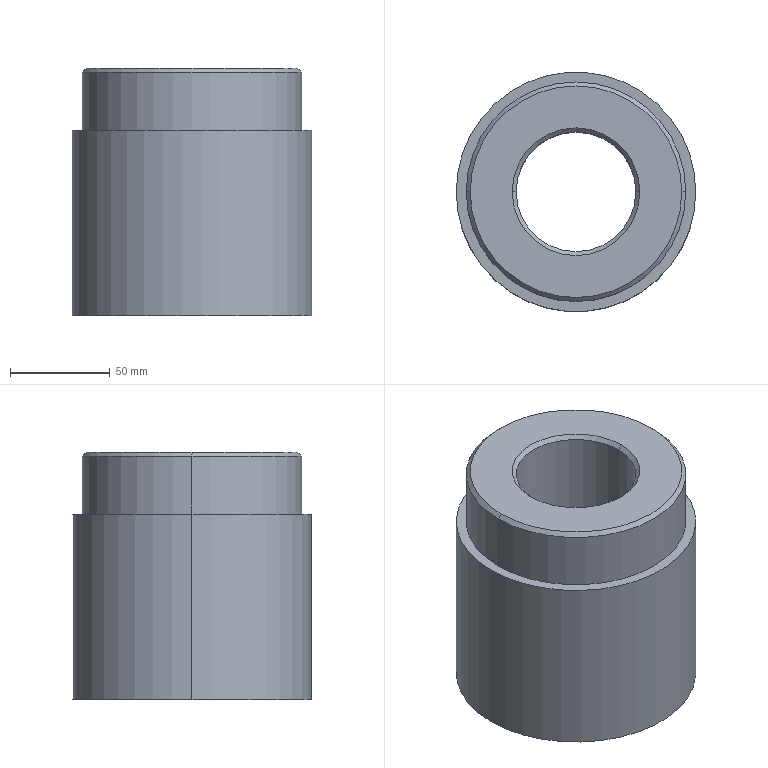Part | SolidWorks | features Chamfer 1, Extrusion 1, ICE 1 | 1 solid | 15 faces | box 120 x 120 x 124 mm | volume 994353 mm3 | cone 6 | cylinder 6 | plane 3 | commonest cylinder face diameters 60 x2 110 x2 120 x2
STEP:
#1=CARTESIAN_POINT('',(-30.,0.,122.));
#2=VERTEX_POINT('',#1);
#3=CARTESIAN_POINT('',(30.,0.,122.));
#4=VERTEX_POINT('',#3);
#5=CARTESIAN_POINT('',(0.,0.,122.));
#6=DIRECTION('',(0.,0.,1.));
#7=DIRECTION('',(1.,0.,0.));
#8=AXIS2_PLACEMENT_3D('',#5,#6,#7);
#9=CIRCLE('',#8,30.);
#10=EDGE_CURVE('',#2,#4,#9,.T.);
#11=ORIENTED_EDGE('',*,*,#10,.F.);
#12=CARTESIAN_POINT('',(-32.,0.,124.));
#13=VERTEX_POINT('',#12);
#14=CARTESIAN_POINT('',(-30.,0.,122.));
#15=DIRECTION('',(-0.7071,0.,0.7071));
#16=VECTOR('',#15,1000.);
#17=LINE('',#14,#16);
#18=EDGE_CURVE('',#2,#13,#17,.T.);
#19=ORIENTED_EDGE('',*,*,#18,.T.);
#20=CARTESIAN_POINT('',(32.,0.,124.));
#21=VERTEX_POINT('',#20);
#22=CARTESIAN_POINT('',(0.,0.,124.));
#23=DIRECTION('',(0.,0.,-1.));
#24=DIRECTION('',(1.,0.,0.));
#25=AXIS2_PLACEMENT_3D('',#22,#23,#24);
#26=CIRCLE('',#25,32.);
#27=EDGE_CURVE('',#21,#13,#26,.T.);
#28=ORIENTED_EDGE('',*,*,#27,.F.);
#29=CARTESIAN_POINT('',(30.,0.,122.));
#30=DIRECTION('',(0.7071,0.,0.7071));
#31=VECTOR('',#30,1000.);
#32=LINE('',#29,#31);
#33=EDGE_CURVE('',#4,#21,#32,.T.);
#34=ORIENTED_EDGE('',*,*,#33,.F.);
#35=EDGE_LOOP('',(#11,#19,#28,#34));
#36=FACE_OUTER_BOUND('',#35,.T.);
#37=CARTESIAN_POINT('',(0.,0.,122.));
#38=DIRECTION('',(0.,0.,1.));
#39=DIRECTION('',(1.,0.,0.));
#40=AXIS2_PLACEMENT_3D('',#37,#38,#39);
#41=CONICAL_SURFACE('',#40,30.,0.7854);
#42=ADVANCED_FACE('',(#36),#41,.F.);
#43=CARTESIAN_POINT('',(53.,0.,124.));
#44=VERTEX_POINT('',#43);
#45=CARTESIAN_POINT('',(-53.,0.,124.));
#46=VERTEX_POINT('',#45);
#47=CARTESIAN_POINT('',(0.,0.,124.));
#48=DIRECTION('',(0.,0.,1.));
#49=DIRECTION('',(1.,0.,0.));
#50=AXIS2_PLACEMENT_3D('',#47,#48,#49);
#51=CIRCLE('',#50,53.);
#52=EDGE_CURVE('',#44,#46,#51,.T.);
#53=ORIENTED_EDGE('',*,*,#52,.F.);
#54=CARTESIAN_POINT('',(55.,0.,122.));
#55=VERTEX_POINT('',#54);
#56=CARTESIAN_POINT('',(53.,0.,124.));
#57=DIRECTION('',(0.7071,0.,-0.7071));
#58=VECTOR('',#57,1000.);
#59=LINE('',#56,#58);
#60=EDGE_CURVE('',#44,#55,#59,.T.);
#61=ORIENTED_EDGE('',*,*,#60,.T.);
#62=CARTESIAN_POINT('',(-55.,0.,122.));
#63=VERTEX_POINT('',#62);
#64=CARTESIAN_POINT('',(0.,0.,122.));
#65=DIRECTION('',(0.,0.,-1.));
#66=DIRECTION('',(1.,0.,0.));
#67=AXIS2_PLACEMENT_3D('',#64,#65,#66);
#68=CIRCLE('',#67,55.);
#69=EDGE_CURVE('',#63,#55,#68,.T.);
#70=ORIENTED_EDGE('',*,*,#69,.F.);
#71=CARTESIAN_POINT('',(-53.,0.,124.));
#72=DIRECTION('',(-0.7071,0.,-0.7071));
#73=VECTOR('',#72,1000.);
#74=LINE('',#71,#73);
#75=EDGE_CURVE('',#46,#63,#74,.T.);
#76=ORIENTED_EDGE('',*,*,#75,.F.);
#77=EDGE_LOOP('',(#53,#61,#70,#76));
#78=FACE_OUTER_BOUND('',#77,.T.);
#79=CARTESIAN_POINT('',(0.,0.,124.));
#80=DIRECTION('',(0.,0.,-1.));
#81=DIRECTION('',(-1.,0.,0.));
#82=AXIS2_PLACEMENT_3D('',#79,#80,#81);
#83=CONICAL_SURFACE('',#82,53.,0.7854);
#84=ADVANCED_FACE('',(#78),#83,.T.);
#85=CARTESIAN_POINT('',(30.,0.,2.));
#86=VERTEX_POINT('',#85);
#87=CARTESIAN_POINT('',(-30.,0.,2.));
#88=VERTEX_POINT('',#87);
#89=CARTESIAN_POINT('',(0.,0.,2.));
#90=DIRECTION('',(0.,0.,-1.));
#91=DIRECTION('',(1.,0.,0.));
#92=AXIS2_PLACEMENT_3D('',#89,#90,#91);
#93=CIRCLE('',#92,30.);
#94=EDGE_CURVE('',#86,#88,#93,.T.);
#95=ORIENTED_EDGE('',*,*,#94,.F.);
#96=CARTESIAN_POINT('',(32.,0.,0.));
#97=VERTEX_POINT('',#96);
#98=CARTESIAN_POINT('',(32.,0.,0.));
#99=DIRECTION('',(0.7071,0.,-0.7071));
#100=VECTOR('',#99,1000.);
#101=LINE('',#98,#100);
#102=EDGE_CURVE('',#86,#97,#101,.T.);
#103=ORIENTED_EDGE('',*,*,#102,.T.);
#104=CARTESIAN_POINT('',(-32.,0.,0.));
#105=VERTEX_POINT('',#104);
#106=CARTESIAN_POINT('',(0.,0.,0.));
#107=DIRECTION('',(0.,0.,1.));
#108=DIRECTION('',(1.,0.,0.));
#109=AXIS2_PLACEMENT_3D('',#106,#107,#108);
#110=CIRCLE('',#109,32.);
#111=EDGE_CURVE('',#105,#97,#110,.T.);
#112=ORIENTED_EDGE('',*,*,#111,.F.);
#113=CARTESIAN_POINT('',(-32.,0.,0.));
#114=DIRECTION('',(-0.7071,0.,-0.7071));
#115=VECTOR('',#114,1000.);
#116=LINE('',#113,#115);
#117=EDGE_CURVE('',#88,#105,#116,.T.);
#118=ORIENTED_EDGE('',*,*,#117,.F.);
#119=EDGE_LOOP('',(#95,#103,#112,#118));
#120=FACE_OUTER_BOUND('',#119,.T.);
#121=CARTESIAN_POINT('',(0.,0.,0.));
#122=DIRECTION('',(0.,0.,-1.));
#123=DIRECTION('',(-1.,0.,0.));
#124=AXIS2_PLACEMENT_3D('',#121,#122,#123);
#125=CONICAL_SURFACE('',#124,32.,0.7854);
#126=ADVANCED_FACE('',(#120),#125,.F.);
#127=CARTESIAN_POINT('',(55.,0.,93.));
#128=VERTEX_POINT('',#127);
#129=CARTESIAN_POINT('',(-55.,0.,93.));
#130=VERTEX_POINT('',#129);
#131=CARTESIAN_POINT('',(0.,0.,93.));
#132=DIRECTION('',(0.,0.,1.));
#133=DIRECTION('',(1.,0.,0.));
#134=AXIS2_PLACEMENT_3D('',#131,#132,#133);
#135=CIRCLE('',#134,55.);
#136=EDGE_CURVE('',#128,#130,#135,.T.);
#137=ORIENTED_EDGE('',*,*,#136,.T.);
#138=CARTESIAN_POINT('',(-55.,0.,93.));
#139=DIRECTION('',(0.,0.,1.));
#140=VECTOR('',#139,1000.);
#141=LINE('',#138,#140);
#142=EDGE_CURVE('',#130,#63,#141,.T.);
#143=ORIENTED_EDGE('',*,*,#142,.T.);
#144=ORIENTED_EDGE('',*,*,#69,.T.);
#145=CARTESIAN_POINT('',(55.,0.,93.));
#146=DIRECTION('',(0.,0.,1.));
#147=VECTOR('',#146,1000.);
#148=LINE('',#145,#147);
#149=EDGE_CURVE('',#128,#55,#148,.T.);
#150=ORIENTED_EDGE('',*,*,#149,.F.);
#151=EDGE_LOOP('',(#137,#143,#144,#150));
#152=FACE_OUTER_BOUND('',#151,.T.);
#153=CARTESIAN_POINT('',(0.,0.,93.));
#154=DIRECTION('',(0.,0.,1.));
#155=DIRECTION('',(1.,0.,0.));
#156=AXIS2_PLACEMENT_3D('',#153,#154,#155);
#157=CYLINDRICAL_SURFACE('',#156,55.);
#158=ADVANCED_FACE('',(#152),#157,.T.);
#159=ORIENTED_EDGE('',*,*,#10,.T.);
#160=CARTESIAN_POINT('',(30.,0.,124.));
#161=DIRECTION('',(0.,0.,-1.));
#162=VECTOR('',#161,1000.);
#163=LINE('',#160,#162);
#164=EDGE_CURVE('',#4,#86,#163,.T.);
#165=ORIENTED_EDGE('',*,*,#164,.T.);
#166=ORIENTED_EDGE('',*,*,#94,.T.);
#167=CARTESIAN_POINT('',(-30.,0.,124.));
#168=DIRECTION('',(0.,0.,-1.));
#169=VECTOR('',#168,1000.);
#170=LINE('',#167,#169);
#171=EDGE_CURVE('',#2,#88,#170,.T.);
#172=ORIENTED_EDGE('',*,*,#171,.F.);
#173=EDGE_LOOP('',(#159,#165,#166,#172));
#174=FACE_OUTER_BOUND('',#173,.T.);
#175=CARTESIAN_POINT('',(0.,0.,124.));
#176=DIRECTION('',(0.,0.,-1.));
#177=DIRECTION('',(-1.,0.,0.));
#178=AXIS2_PLACEMENT_3D('',#175,#176,#177);
#179=CYLINDRICAL_SURFACE('',#178,30.);
#180=ADVANCED_FACE('',(#174),#179,.F.);
#181=CARTESIAN_POINT('',(60.,0.,93.));
#182=VERTEX_POINT('',#181);
#183=CARTESIAN_POINT('',(-60.,0.,93.));
#184=VERTEX_POINT('',#183);
#185=CARTESIAN_POINT('',(0.,0.,93.));
#186=DIRECTION('',(0.,0.,1.));
#187=DIRECTION('',(1.,0.,0.));
#188=AXIS2_PLACEMENT_3D('',#185,#186,#187);
#189=CIRCLE('',#188,60.);
#190=EDGE_CURVE('',#182,#184,#189,.T.);
#191=ORIENTED_EDGE('',*,*,#190,.F.);
#192=CARTESIAN_POINT('',(60.,0.,0.));
#193=VERTEX_POINT('',#192);
#194=CARTESIAN_POINT('',(60.,0.,124.));
#195=DIRECTION('',(0.,0.,-1.));
#196=VECTOR('',#195,1000.);
#197=LINE('',#194,#196);
#198=EDGE_CURVE('',#182,#193,#197,.T.);
#199=ORIENTED_EDGE('',*,*,#198,.T.);
#200=CARTESIAN_POINT('',(-60.,0.,0.));
#201=VERTEX_POINT('',#200);
#202=CARTESIAN_POINT('',(0.,0.,0.));
#203=DIRECTION('',(0.,0.,1.));
#204=DIRECTION('',(1.,0.,0.));
#205=AXIS2_PLACEMENT_3D('',#202,#203,#204);
#206=CIRCLE('',#205,60.);
#207=EDGE_CURVE('',#193,#201,#206,.T.);
#208=ORIENTED_EDGE('',*,*,#207,.T.);
#209=CARTESIAN_POINT('',(-60.,0.,124.));
#210=DIRECTION('',(0.,0.,-1.));
#211=VECTOR('',#210,1000.);
#212=LINE('',#209,#211);
#213=EDGE_CURVE('',#184,#201,#212,.T.);
#214=ORIENTED_EDGE('',*,*,#213,.F.);
#215=EDGE_LOOP('',(#191,#199,#208,#214));
#216=FACE_OUTER_BOUND('',#215,.T.);
#217=CARTESIAN_POINT('',(0.,0.,124.));
#218=DIRECTION('',(0.,0.,-1.));
#219=DIRECTION('',(-1.,0.,0.));
#220=AXIS2_PLACEMENT_3D('',#217,#218,#219);
#221=CYLINDRICAL_SURFACE('',#220,60.);
#222=ADVANCED_FACE('',(#216),#221,.T.);
#223=CARTESIAN_POINT('',(0.,0.,124.));
#224=DIRECTION('',(0.,0.,1.));
#225=DIRECTION('',(1.,0.,0.));
#226=AXIS2_PLACEMENT_3D('',#223,#224,#225);
#227=CIRCLE('',#226,53.);
#228=EDGE_CURVE('',#46,#44,#227,.T.);
#229=ORIENTED_EDGE('',*,*,#228,.T.);
#230=ORIENTED_EDGE('',*,*,#52,.T.);
#231=EDGE_LOOP('',(#229,#230));
#232=FACE_OUTER_BOUND('',#231,.T.);
#233=ORIENTED_EDGE('',*,*,#27,.T.);
#234=CARTESIAN_POINT('',(0.,0.,124.));
#235=DIRECTION('',(0.,0.,-1.));
#236=DIRECTION('',(1.,0.,0.));
#237=AXIS2_PLACEMENT_3D('',#234,#235,#236);
#238=CIRCLE('',#237,32.);
#239=EDGE_CURVE('',#13,#21,#238,.T.);
#240=ORIENTED_EDGE('',*,*,#239,.T.);
#241=EDGE_LOOP('',(#233,#240));
#242=FACE_BOUND('',#241,.T.);
#243=CARTESIAN_POINT('',(0.,0.,124.));
#244=DIRECTION('',(0.,0.,1.));
#245=DIRECTION('',(1.,0.,0.));
#246=AXIS2_PLACEMENT_3D('',#243,#244,#245);
#247=PLANE('',#246);
#248=ADVANCED_FACE('',(#232,#242),#247,.T.);
#249=ORIENTED_EDGE('',*,*,#198,.F.);
#250=CARTESIAN_POINT('',(0.,0.,93.));
#251=DIRECTION('',(0.,0.,1.));
#252=DIRECTION('',(1.,0.,0.));
#253=AXIS2_PLACEMENT_3D('',#250,#251,#252);
#254=CIRCLE('',#253,60.);
#255=EDGE_CURVE('',#184,#182,#254,.T.);
#256=ORIENTED_EDGE('',*,*,#255,.F.);
#257=ORIENTED_EDGE('',*,*,#213,.T.);
#258=CARTESIAN_POINT('',(0.,0.,0.));
#259=DIRECTION('',(0.,0.,1.));
#260=DIRECTION('',(1.,0.,0.));
#261=AXIS2_PLACEMENT_3D('',#258,#259,#260);
#262=CIRCLE('',#261,60.);
#263=EDGE_CURVE('',#201,#193,#262,.T.);
#264=ORIENTED_EDGE('',*,*,#263,.T.);
#265=EDGE_LOOP('',(#249,#256,#257,#264));
#266=FACE_OUTER_BOUND('',#265,.T.);
#267=CARTESIAN_POINT('',(0.,0.,124.));
#268=DIRECTION('',(0.,0.,-1.));
#269=DIRECTION('',(-1.,0.,0.));
#270=AXIS2_PLACEMENT_3D('',#267,#268,#269);
#271=CYLINDRICAL_SURFACE('',#270,60.);
#272=ADVANCED_FACE('',(#266),#271,.T.);
#273=ORIENTED_EDGE('',*,*,#111,.T.);
#274=CARTESIAN_POINT('',(0.,0.,0.));
#275=DIRECTION('',(0.,0.,1.));
#276=DIRECTION('',(1.,0.,0.));
#277=AXIS2_PLACEMENT_3D('',#274,#275,#276);
#278=CIRCLE('',#277,32.);
#279=EDGE_CURVE('',#97,#105,#278,.T.);
#280=ORIENTED_EDGE('',*,*,#279,.T.);
#281=EDGE_LOOP('',(#273,#280));
#282=FACE_BOUND('',#281,.T.);
#283=ORIENTED_EDGE('',*,*,#263,.F.);
#284=ORIENTED_EDGE('',*,*,#207,.F.);
#285=EDGE_LOOP('',(#283,#284));
#286=FACE_OUTER_BOUND('',#285,.T.);
#287=CARTESIAN_POINT('',(0.,0.,0.));
#288=DIRECTION('',(0.,0.,1.));
#289=DIRECTION('',(1.,0.,0.));
#290=AXIS2_PLACEMENT_3D('',#287,#288,#289);
#291=PLANE('',#290);
#292=ADVANCED_FACE('',(#282,#286),#291,.F.);
#293=ORIENTED_EDGE('',*,*,#164,.F.);
#294=CARTESIAN_POINT('',(0.,0.,122.));
#295=DIRECTION('',(0.,0.,1.));
#296=DIRECTION('',(1.,0.,0.));
#297=AXIS2_PLACEMENT_3D('',#294,#295,#296);
#298=CIRCLE('',#297,30.);
#299=EDGE_CURVE('',#4,#2,#298,.T.);
#300=ORIENTED_EDGE('',*,*,#299,.T.);
#301=ORIENTED_EDGE('',*,*,#171,.T.);
#302=CARTESIAN_POINT('',(0.,0.,2.));
#303=DIRECTION('',(0.,0.,-1.));
#304=DIRECTION('',(1.,0.,0.));
#305=AXIS2_PLACEMENT_3D('',#302,#303,#304);
#306=CIRCLE('',#305,30.);
#307=EDGE_CURVE('',#88,#86,#306,.T.);
#308=ORIENTED_EDGE('',*,*,#307,.T.);
#309=EDGE_LOOP('',(#293,#300,#301,#308));
#310=FACE_OUTER_BOUND('',#309,.T.);
#311=CARTESIAN_POINT('',(0.,0.,124.));
#312=DIRECTION('',(0.,0.,-1.));
#313=DIRECTION('',(-1.,0.,0.));
#314=AXIS2_PLACEMENT_3D('',#311,#312,#313);
#315=CYLINDRICAL_SURFACE('',#314,30.);
#316=ADVANCED_FACE('',(#310),#315,.F.);
#317=ORIENTED_EDGE('',*,*,#136,.F.);
#318=CARTESIAN_POINT('',(0.,0.,93.));
#319=DIRECTION('',(0.,0.,1.));
#320=DIRECTION('',(1.,0.,0.));
#321=AXIS2_PLACEMENT_3D('',#318,#319,#320);
#322=CIRCLE('',#321,55.);
#323=EDGE_CURVE('',#130,#128,#322,.T.);
#324=ORIENTED_EDGE('',*,*,#323,.F.);
#325=EDGE_LOOP('',(#317,#324));
#326=FACE_BOUND('',#325,.T.);
#327=ORIENTED_EDGE('',*,*,#255,.T.);
#328=ORIENTED_EDGE('',*,*,#190,.T.);
#329=EDGE_LOOP('',(#327,#328));
#330=FACE_OUTER_BOUND('',#329,.T.);
#331=CARTESIAN_POINT('',(0.,0.,93.));
#332=DIRECTION('',(0.,0.,1.));
#333=DIRECTION('',(1.,0.,0.));
#334=AXIS2_PLACEMENT_3D('',#331,#332,#333);
#335=PLANE('',#334);
#336=ADVANCED_FACE('',(#326,#330),#335,.T.);
#337=ORIENTED_EDGE('',*,*,#142,.F.);
#338=ORIENTED_EDGE('',*,*,#323,.T.);
#339=ORIENTED_EDGE('',*,*,#149,.T.);
#340=CARTESIAN_POINT('',(0.,0.,122.));
#341=DIRECTION('',(0.,0.,-1.));
#342=DIRECTION('',(1.,0.,0.));
#343=AXIS2_PLACEMENT_3D('',#340,#341,#342);
#344=CIRCLE('',#343,55.);
#345=EDGE_CURVE('',#55,#63,#344,.T.);
#346=ORIENTED_EDGE('',*,*,#345,.T.);
#347=EDGE_LOOP('',(#337,#338,#339,#346));
#348=FACE_OUTER_BOUND('',#347,.T.);
#349=CARTESIAN_POINT('',(0.,0.,93.));
#350=DIRECTION('',(0.,0.,1.));
#351=DIRECTION('',(1.,0.,0.));
#352=AXIS2_PLACEMENT_3D('',#349,#350,#351);
#353=CYLINDRICAL_SURFACE('',#352,55.);
#354=ADVANCED_FACE('',(#348),#353,.T.);
#355=ORIENTED_EDGE('',*,*,#102,.F.);
#356=ORIENTED_EDGE('',*,*,#307,.F.);
#357=ORIENTED_EDGE('',*,*,#117,.T.);
#358=ORIENTED_EDGE('',*,*,#279,.F.);
#359=EDGE_LOOP('',(#355,#356,#357,#358));
#360=FACE_OUTER_BOUND('',#359,.T.);
#361=CARTESIAN_POINT('',(0.,0.,0.));
#362=DIRECTION('',(0.,0.,-1.));
#363=DIRECTION('',(-1.,0.,0.));
#364=AXIS2_PLACEMENT_3D('',#361,#362,#363);
#365=CONICAL_SURFACE('',#364,32.,0.7854);
#366=ADVANCED_FACE('',(#360),#365,.F.);
#367=ORIENTED_EDGE('',*,*,#60,.F.);
#368=ORIENTED_EDGE('',*,*,#228,.F.);
#369=ORIENTED_EDGE('',*,*,#75,.T.);
#370=ORIENTED_EDGE('',*,*,#345,.F.);
#371=EDGE_LOOP('',(#367,#368,#369,#370));
#372=FACE_OUTER_BOUND('',#371,.T.);
#373=CARTESIAN_POINT('',(0.,0.,124.));
#374=DIRECTION('',(0.,0.,-1.));
#375=DIRECTION('',(-1.,0.,0.));
#376=AXIS2_PLACEMENT_3D('',#373,#374,#375);
#377=CONICAL_SURFACE('',#376,53.,0.7854);
#378=ADVANCED_FACE('',(#372),#377,.T.);
#379=ORIENTED_EDGE('',*,*,#18,.F.);
#380=ORIENTED_EDGE('',*,*,#299,.F.);
#381=ORIENTED_EDGE('',*,*,#33,.T.);
#382=ORIENTED_EDGE('',*,*,#239,.F.);
#383=EDGE_LOOP('',(#379,#380,#381,#382));
#384=FACE_OUTER_BOUND('',#383,.T.);
#385=CARTESIAN_POINT('',(0.,0.,122.));
#386=DIRECTION('',(0.,0.,1.));
#387=DIRECTION('',(1.,0.,0.));
#388=AXIS2_PLACEMENT_3D('',#385,#386,#387);
#389=CONICAL_SURFACE('',#388,30.,0.7854);
#390=ADVANCED_FACE('',(#384),#389,.F.);
#391=CLOSED_SHELL('',(#42,#84,#126,#158,#180,#222,#248,#272,#292,#316,#336,#354,#366,#378,#390));
#392=MANIFOLD_SOLID_BREP('',#391);
#393=CARTESIAN_POINT('',(0.,0.,0.));
#394=DIRECTION('',(0.,0.,1.));
#395=DIRECTION('',(1.,0.,0.));
#396=AXIS2_PLACEMENT_3D('',#393,#394,#395);
#397=(LENGTH_UNIT()NAMED_UNIT(*)SI_UNIT(.MILLI.,.METRE.));
#398=UNCERTAINTY_MEASURE_WITH_UNIT(LENGTH_MEASURE(0.00001),#397,'','');
#399=(NAMED_UNIT(*)PLANE_ANGLE_UNIT()SI_UNIT($,.RADIAN.));
#400=(NAMED_UNIT(*)SI_UNIT($,.STERADIAN.)SOLID_ANGLE_UNIT());
#401=(GEOMETRIC_REPRESENTATION_CONTEXT(3)GLOBAL_UNCERTAINTY_ASSIGNED_CONTEXT((#398))GLOBAL_UNIT_ASSIGNED_CONTEXT((#397,#399,#400))REPRESENTATION_CONTEXT('',''));
#402=ADVANCED_BREP_SHAPE_REPRESENTATION('',(#392,#396),#401);